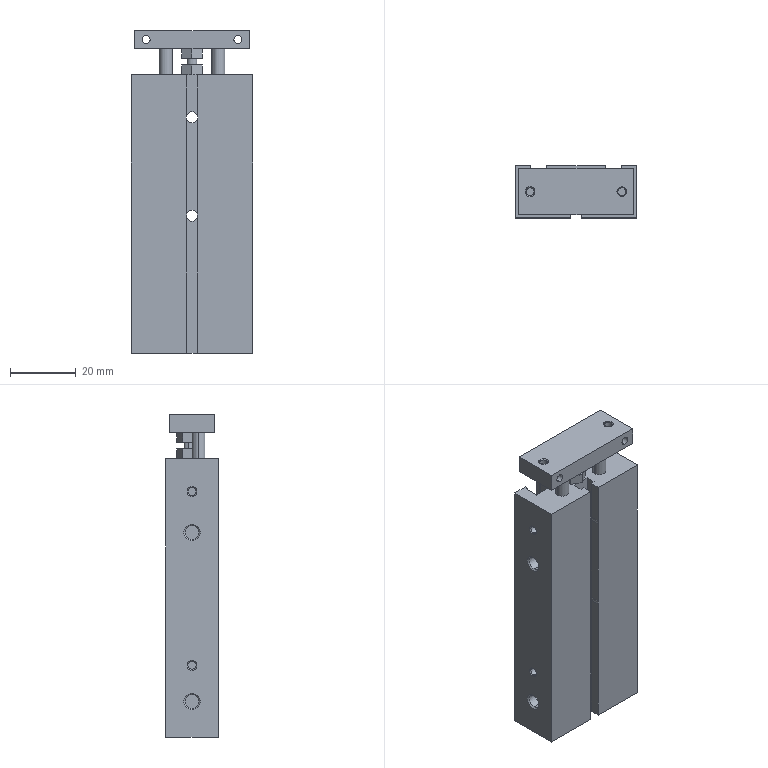Part | STEP file | Mount electronic clip cylinder CXSM6-40(0) | 1 solid | 142 faces | box 37 x 16 x 98.5 mm | volume 44688 mm3 | plane 66 | cylinder 52 | cone 24 | commonest cylinder face diameters 2.46 x24 3.4 x8 4.13 x8 3 x4 4 x4 6.5 x4